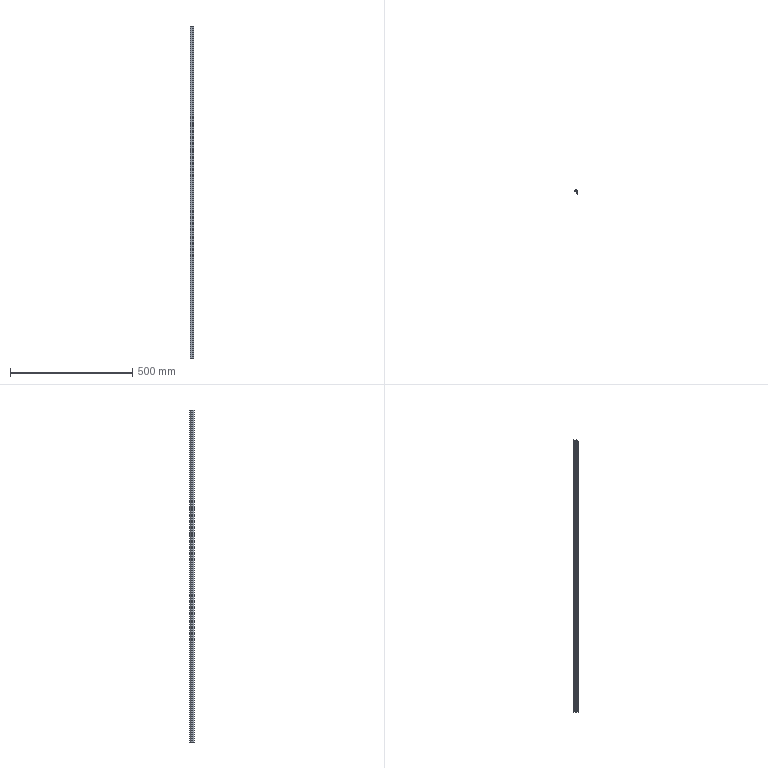Part | SolidWorks | features BaseBody 1, ICE 1, MoveFace 1 | 1 solid | 27 faces | box 14 x 20.3 x 1358 mm | volume 69144 mm3 | plane 20 | cylinder 7 | commonest cylinder face diameters 0.387 x2 0.8 x2 0.4 x1 20 x1 22 x1
STEP:
#1=CARTESIAN_POINT('',(-5.304,-0.625,200.));
#2=VERTEX_POINT('',#1);
#3=CARTESIAN_POINT('',(-5.449,-0.8125,200.));
#4=VERTEX_POINT('',#3);
#5=CARTESIAN_POINT('',(-5.255,-0.8125,200.));
#6=DIRECTION('',(0.,0.,1.));
#7=DIRECTION('',(-1.,0.,0.));
#8=AXIS2_PLACEMENT_3D('',#5,#6,#7);
#9=CIRCLE('',#8,0.1937);
#10=EDGE_CURVE('',#2,#4,#9,.T.);
#11=ORIENTED_EDGE('',*,*,#10,.T.);
#12=CARTESIAN_POINT('',(-5.449,-0.8125,-1158.));
#13=VERTEX_POINT('',#12);
#14=CARTESIAN_POINT('',(-5.449,-0.8125,230.));
#15=DIRECTION('',(0.,0.,-1.));
#16=VECTOR('',#15,1000.);
#17=LINE('',#14,#16);
#18=EDGE_CURVE('',#4,#13,#17,.T.);
#19=ORIENTED_EDGE('',*,*,#18,.T.);
#20=CARTESIAN_POINT('',(-5.304,-0.625,-1158.));
#21=VERTEX_POINT('',#20);
#22=CARTESIAN_POINT('',(-5.255,-0.8125,-1158.));
#23=DIRECTION('',(0.,0.,-1.));
#24=DIRECTION('',(1.,0.,0.));
#25=AXIS2_PLACEMENT_3D('',#22,#23,#24);
#26=CIRCLE('',#25,0.1937);
#27=EDGE_CURVE('',#13,#21,#26,.T.);
#28=ORIENTED_EDGE('',*,*,#27,.T.);
#29=CARTESIAN_POINT('',(-5.304,-0.625,230.));
#30=DIRECTION('',(0.,0.,-1.));
#31=VECTOR('',#30,1000.);
#32=LINE('',#29,#31);
#33=EDGE_CURVE('',#2,#21,#32,.T.);
#34=ORIENTED_EDGE('',*,*,#33,.F.);
#35=EDGE_LOOP('',(#11,#19,#28,#34));
#36=FACE_OUTER_BOUND('',#35,.T.);
#37=CARTESIAN_POINT('',(-5.255,-0.8125,230.));
#38=DIRECTION('',(0.,0.,-1.));
#39=DIRECTION('',(-1.,0.,0.));
#40=AXIS2_PLACEMENT_3D('',#37,#38,#39);
#41=CYLINDRICAL_SURFACE('',#40,0.1937);
#42=ADVANCED_FACE('',(#36),#41,.F.);
#43=CARTESIAN_POINT('',(5.,-1.,-1158.));
#44=VERTEX_POINT('',#43);
#45=CARTESIAN_POINT('',(5.,-14.3,-1158.));
#46=VERTEX_POINT('',#45);
#47=CARTESIAN_POINT('',(5.,29.623,-1158.));
#48=DIRECTION('',(0.,-1.,0.));
#49=VECTOR('',#48,1000.);
#50=LINE('',#47,#49);
#51=EDGE_CURVE('',#44,#46,#50,.T.);
#52=ORIENTED_EDGE('',*,*,#51,.F.);
#53=CARTESIAN_POINT('',(5.,-1.,200.));
#54=VERTEX_POINT('',#53);
#55=CARTESIAN_POINT('',(5.,-1.,230.));
#56=DIRECTION('',(0.,0.,-1.));
#57=VECTOR('',#56,1000.);
#58=LINE('',#55,#57);
#59=EDGE_CURVE('',#54,#44,#58,.T.);
#60=ORIENTED_EDGE('',*,*,#59,.F.);
#61=CARTESIAN_POINT('',(5.,-14.3,200.));
#62=VERTEX_POINT('',#61);
#63=CARTESIAN_POINT('',(5.,-14.3,200.));
#64=DIRECTION('',(0.,1.,0.));
#65=VECTOR('',#64,1000.);
#66=LINE('',#63,#65);
#67=EDGE_CURVE('',#62,#54,#66,.T.);
#68=ORIENTED_EDGE('',*,*,#67,.F.);
#69=CARTESIAN_POINT('',(5.,-14.3,230.));
#70=DIRECTION('',(0.,0.,1.));
#71=VECTOR('',#70,1000.);
#72=LINE('',#69,#71);
#73=EDGE_CURVE('',#46,#62,#72,.T.);
#74=ORIENTED_EDGE('',*,*,#73,.F.);
#75=EDGE_LOOP('',(#52,#60,#68,#74));
#76=FACE_OUTER_BOUND('',#75,.T.);
#77=CARTESIAN_POINT('',(5.,-14.3,230.));
#78=DIRECTION('',(-1.,0.,0.));
#79=DIRECTION('',(0.,0.,1.));
#80=AXIS2_PLACEMENT_3D('',#77,#78,#79);
#81=PLANE('',#80);
#82=ADVANCED_FACE('',(#76),#81,.F.);
#83=CARTESIAN_POINT('',(-9.,-2.,-1158.));
#84=VERTEX_POINT('',#83);
#85=CARTESIAN_POINT('',(-9.,-2.,200.));
#86=VERTEX_POINT('',#85);
#87=CARTESIAN_POINT('',(-9.,-2.,230.));
#88=DIRECTION('',(0.,0.,1.));
#89=VECTOR('',#88,1000.);
#90=LINE('',#87,#89);
#91=EDGE_CURVE('',#84,#86,#90,.T.);
#92=ORIENTED_EDGE('',*,*,#91,.F.);
#93=CARTESIAN_POINT('',(0.9,-2.,-1158.));
#94=VERTEX_POINT('',#93);
#95=CARTESIAN_POINT('',(5.,-2.,-1158.));
#96=DIRECTION('',(-1.,0.,0.));
#97=VECTOR('',#96,1000.);
#98=LINE('',#95,#97);
#99=EDGE_CURVE('',#94,#84,#98,.T.);
#100=ORIENTED_EDGE('',*,*,#99,.F.);
#101=CARTESIAN_POINT('',(0.9,-2.,200.));
#102=VERTEX_POINT('',#101);
#103=CARTESIAN_POINT('',(0.9,-2.,230.));
#104=DIRECTION('',(0.,0.,-1.));
#105=VECTOR('',#104,1000.);
#106=LINE('',#103,#105);
#107=EDGE_CURVE('',#102,#94,#106,.T.);
#108=ORIENTED_EDGE('',*,*,#107,.F.);
#109=CARTESIAN_POINT('',(5.,-2.,200.));
#110=DIRECTION('',(1.,0.,0.));
#111=VECTOR('',#110,1000.);
#112=LINE('',#109,#111);
#113=EDGE_CURVE('',#86,#102,#112,.T.);
#114=ORIENTED_EDGE('',*,*,#113,.F.);
#115=EDGE_LOOP('',(#92,#100,#108,#114));
#116=FACE_OUTER_BOUND('',#115,.T.);
#117=CARTESIAN_POINT('',(-9.,-2.,230.));
#118=DIRECTION('',(0.,1.,0.));
#119=DIRECTION('',(0.,0.,1.));
#120=AXIS2_PLACEMENT_3D('',#117,#118,#119);
#121=PLANE('',#120);
#122=ADVANCED_FACE('',(#116),#121,.F.);
#123=CARTESIAN_POINT('',(4.,-6.,200.));
#124=VERTEX_POINT('',#123);
#125=CARTESIAN_POINT('',(4.,-3.,200.));
#126=VERTEX_POINT('',#125);
#127=CARTESIAN_POINT('',(4.,29.623,200.));
#128=DIRECTION('',(0.,1.,0.));
#129=VECTOR('',#128,1000.);
#130=LINE('',#127,#129);
#131=EDGE_CURVE('',#124,#126,#130,.T.);
#132=ORIENTED_EDGE('',*,*,#131,.F.);
#133=CARTESIAN_POINT('',(1.,-6.,200.));
#134=VERTEX_POINT('',#133);
#135=CARTESIAN_POINT('',(5.,-6.,200.));
#136=DIRECTION('',(1.,0.,0.));
#137=VECTOR('',#136,1000.);
#138=LINE('',#135,#137);
#139=EDGE_CURVE('',#134,#124,#138,.T.);
#140=ORIENTED_EDGE('',*,*,#139,.F.);
#141=CARTESIAN_POINT('',(1.,-6.7,200.));
#142=VERTEX_POINT('',#141);
#143=CARTESIAN_POINT('',(1.,-6.,200.));
#144=DIRECTION('',(0.,-1.,0.));
#145=VECTOR('',#144,1000.);
#146=LINE('',#143,#145);
#147=EDGE_CURVE('',#134,#142,#146,.T.);
#148=ORIENTED_EDGE('',*,*,#147,.T.);
#149=CARTESIAN_POINT('',(-1.7,-6.7,200.));
#150=VERTEX_POINT('',#149);
#151=CARTESIAN_POINT('',(5.,-6.7,200.));
#152=DIRECTION('',(1.,0.,0.));
#153=VECTOR('',#152,1000.);
#154=LINE('',#151,#153);
#155=EDGE_CURVE('',#150,#142,#154,.T.);
#156=ORIENTED_EDGE('',*,*,#155,.F.);
#157=CARTESIAN_POINT('',(-1.7,-7.7,200.));
#158=VERTEX_POINT('',#157);
#159=CARTESIAN_POINT('',(-1.7,-6.7,200.));
#160=DIRECTION('',(0.,-1.,0.));
#161=VECTOR('',#160,1000.);
#162=LINE('',#159,#161);
#163=EDGE_CURVE('',#150,#158,#162,.T.);
#164=ORIENTED_EDGE('',*,*,#163,.T.);
#165=CARTESIAN_POINT('',(4.,-7.7,200.));
#166=VERTEX_POINT('',#165);
#167=CARTESIAN_POINT('',(5.,-7.7,200.));
#168=DIRECTION('',(-1.,0.,0.));
#169=VECTOR('',#168,1000.);
#170=LINE('',#167,#169);
#171=EDGE_CURVE('',#166,#158,#170,.T.);
#172=ORIENTED_EDGE('',*,*,#171,.F.);
#173=CARTESIAN_POINT('',(4.,-14.3,200.));
#174=VERTEX_POINT('',#173);
#175=CARTESIAN_POINT('',(4.,29.623,200.));
#176=DIRECTION('',(0.,1.,0.));
#177=VECTOR('',#176,1000.);
#178=LINE('',#175,#177);
#179=EDGE_CURVE('',#174,#166,#178,.T.);
#180=ORIENTED_EDGE('',*,*,#179,.F.);
#181=CARTESIAN_POINT('',(5.,-14.3,200.));
#182=DIRECTION('',(-1.,0.,0.));
#183=VECTOR('',#182,1000.);
#184=LINE('',#181,#183);
#185=EDGE_CURVE('',#62,#174,#184,.T.);
#186=ORIENTED_EDGE('',*,*,#185,.F.);
#187=ORIENTED_EDGE('',*,*,#67,.T.);
#188=CARTESIAN_POINT('',(-5.207,-1.,200.));
#189=VERTEX_POINT('',#188);
#190=CARTESIAN_POINT('',(5.,-1.,200.));
#191=DIRECTION('',(1.,0.,0.));
#192=VECTOR('',#191,1000.);
#193=LINE('',#190,#192);
#194=EDGE_CURVE('',#189,#54,#193,.T.);
#195=ORIENTED_EDGE('',*,*,#194,.F.);
#196=CARTESIAN_POINT('',(-5.255,-0.8125,200.));
#197=DIRECTION('',(0.,0.,1.));
#198=DIRECTION('',(-1.,0.,0.));
#199=AXIS2_PLACEMENT_3D('',#196,#197,#198);
#200=CIRCLE('',#199,0.1937);
#201=EDGE_CURVE('',#4,#189,#200,.T.);
#202=ORIENTED_EDGE('',*,*,#201,.F.);
#203=ORIENTED_EDGE('',*,*,#10,.F.);
#204=CARTESIAN_POINT('',(-1.368,3.063,200.));
#205=VERTEX_POINT('',#204);
#206=CARTESIAN_POINT('',(-10.628,9.,200.));
#207=DIRECTION('',(0.,0.,1.));
#208=DIRECTION('',(-1.,0.,0.));
#209=AXIS2_PLACEMENT_3D('',#206,#207,#208);
#210=CIRCLE('',#209,11.);
#211=EDGE_CURVE('',#2,#205,#210,.T.);
#212=ORIENTED_EDGE('',*,*,#211,.T.);
#213=CARTESIAN_POINT('',(-1.,2.955,200.));
#214=VERTEX_POINT('',#213);
#215=CARTESIAN_POINT('',(-1.2,2.955,200.));
#216=DIRECTION('',(0.,0.,1.));
#217=DIRECTION('',(-1.,0.,0.));
#218=AXIS2_PLACEMENT_3D('',#215,#216,#217);
#219=CIRCLE('',#218,0.2);
#220=EDGE_CURVE('',#214,#205,#219,.T.);
#221=ORIENTED_EDGE('',*,*,#220,.F.);
#222=CARTESIAN_POINT('',(-1.,1.5,200.));
#223=VERTEX_POINT('',#222);
#224=CARTESIAN_POINT('',(-1.,2.955,200.));
#225=DIRECTION('',(0.,1.,0.));
#226=VECTOR('',#225,1000.);
#227=LINE('',#224,#226);
#228=EDGE_CURVE('',#223,#214,#227,.T.);
#229=ORIENTED_EDGE('',*,*,#228,.F.);
#230=CARTESIAN_POINT('',(0.,1.5,200.));
#231=VERTEX_POINT('',#230);
#232=CARTESIAN_POINT('',(-1.,1.5,200.));
#233=DIRECTION('',(-1.,0.,0.));
#234=VECTOR('',#233,1000.);
#235=LINE('',#232,#234);
#236=EDGE_CURVE('',#231,#223,#235,.T.);
#237=ORIENTED_EDGE('',*,*,#236,.F.);
#238=CARTESIAN_POINT('',(0.,6.,200.));
#239=VERTEX_POINT('',#238);
#240=CARTESIAN_POINT('',(0.,1.5,200.));
#241=DIRECTION('',(0.,-1.,0.));
#242=VECTOR('',#241,1000.);
#243=LINE('',#240,#242);
#244=EDGE_CURVE('',#239,#231,#243,.T.);
#245=ORIENTED_EDGE('',*,*,#244,.F.);
#246=CARTESIAN_POINT('',(-0.8,6.,200.));
#247=VERTEX_POINT('',#246);
#248=CARTESIAN_POINT('',(0.,6.,200.));
#249=DIRECTION('',(1.,0.,0.));
#250=VECTOR('',#249,1000.);
#251=LINE('',#248,#250);
#252=EDGE_CURVE('',#247,#239,#251,.T.);
#253=ORIENTED_EDGE('',*,*,#252,.F.);
#254=CARTESIAN_POINT('',(-1.178,5.731,200.));
#255=VERTEX_POINT('',#254);
#256=CARTESIAN_POINT('',(-0.8,5.6,200.));
#257=DIRECTION('',(0.,0.,1.));
#258=DIRECTION('',(-1.,0.,0.));
#259=AXIS2_PLACEMENT_3D('',#256,#257,#258);
#260=CIRCLE('',#259,0.4);
#261=EDGE_CURVE('',#247,#255,#260,.T.);
#262=ORIENTED_EDGE('',*,*,#261,.T.);
#263=CARTESIAN_POINT('',(-8.678,-0.8077,200.));
#264=VERTEX_POINT('',#263);
#265=CARTESIAN_POINT('',(-10.628,9.,200.));
#266=DIRECTION('',(0.,0.,1.));
#267=DIRECTION('',(-1.,0.,0.));
#268=AXIS2_PLACEMENT_3D('',#265,#266,#267);
#269=CIRCLE('',#268,10.);
#270=EDGE_CURVE('',#264,#255,#269,.T.);
#271=ORIENTED_EDGE('',*,*,#270,.F.);
#272=CARTESIAN_POINT('',(-9.,-1.2,200.));
#273=VERTEX_POINT('',#272);
#274=CARTESIAN_POINT('',(-8.6,-1.2,200.));
#275=DIRECTION('',(0.,0.,1.));
#276=DIRECTION('',(-1.,0.,0.));
#277=AXIS2_PLACEMENT_3D('',#274,#275,#276);
#278=CIRCLE('',#277,0.4);
#279=EDGE_CURVE('',#264,#273,#278,.T.);
#280=ORIENTED_EDGE('',*,*,#279,.T.);
#281=CARTESIAN_POINT('',(-9.,8.,200.));
#282=DIRECTION('',(0.,-1.,0.));
#283=VECTOR('',#282,1000.);
#284=LINE('',#281,#283);
#285=EDGE_CURVE('',#273,#86,#284,.T.);
#286=ORIENTED_EDGE('',*,*,#285,.T.);
#287=ORIENTED_EDGE('',*,*,#113,.T.);
#288=CARTESIAN_POINT('',(0.9,-3.,200.));
#289=VERTEX_POINT('',#288);
#290=CARTESIAN_POINT('',(0.9,29.623,200.));
#291=DIRECTION('',(0.,1.,0.));
#292=VECTOR('',#291,1000.);
#293=LINE('',#290,#292);
#294=EDGE_CURVE('',#289,#102,#293,.T.);
#295=ORIENTED_EDGE('',*,*,#294,.F.);
#296=CARTESIAN_POINT('',(5.,-3.,200.));
#297=DIRECTION('',(-1.,0.,0.));
#298=VECTOR('',#297,1000.);
#299=LINE('',#296,#298);
#300=EDGE_CURVE('',#126,#289,#299,.T.);
#301=ORIENTED_EDGE('',*,*,#300,.F.);
#302=EDGE_LOOP('',(#132,#140,#148,#156,#164,#172,#180,#186,#187,#195,#202,#203,#212,#221,#229,#237,#245,#253,#262,#271,#280,#286,#287,#295,#301));
#303=FACE_OUTER_BOUND('',#302,.T.);
#304=CARTESIAN_POINT('',(5.,29.623,200.));
#305=DIRECTION('',(0.,0.,-1.));
#306=DIRECTION('',(-1.,0.,0.));
#307=AXIS2_PLACEMENT_3D('',#304,#305,#306);
#308=PLANE('',#307);
#309=ADVANCED_FACE('',(#303),#308,.F.);
#310=ORIENTED_EDGE('',*,*,#185,.T.);
#311=CARTESIAN_POINT('',(4.,-14.3,-1158.));
#312=VERTEX_POINT('',#311);
#313=CARTESIAN_POINT('',(4.,-14.3,230.));
#314=DIRECTION('',(0.,0.,1.));
#315=VECTOR('',#314,1000.);
#316=LINE('',#313,#315);
#317=EDGE_CURVE('',#312,#174,#316,.T.);
#318=ORIENTED_EDGE('',*,*,#317,.F.);
#319=CARTESIAN_POINT('',(5.,-14.3,-1158.));
#320=DIRECTION('',(-1.,0.,0.));
#321=VECTOR('',#320,1000.);
#322=LINE('',#319,#321);
#323=EDGE_CURVE('',#46,#312,#322,.T.);
#324=ORIENTED_EDGE('',*,*,#323,.F.);
#325=ORIENTED_EDGE('',*,*,#73,.T.);
#326=EDGE_LOOP('',(#310,#318,#324,#325));
#327=FACE_OUTER_BOUND('',#326,.T.);
#328=CARTESIAN_POINT('',(4.,-14.3,230.));
#329=DIRECTION('',(0.,1.,0.));
#330=DIRECTION('',(0.,0.,1.));
#331=AXIS2_PLACEMENT_3D('',#328,#329,#330);
#332=PLANE('',#331);
#333=ADVANCED_FACE('',(#327),#332,.F.);
#334=ORIENTED_EDGE('',*,*,#51,.T.);
#335=ORIENTED_EDGE('',*,*,#323,.T.);
#336=CARTESIAN_POINT('',(4.,-7.7,-1158.));
#337=VERTEX_POINT('',#336);
#338=CARTESIAN_POINT('',(4.,-7.7,-1158.));
#339=DIRECTION('',(0.,-1.,0.));
#340=VECTOR('',#339,1000.);
#341=LINE('',#338,#340);
#342=EDGE_CURVE('',#337,#312,#341,.T.);
#343=ORIENTED_EDGE('',*,*,#342,.F.);
#344=CARTESIAN_POINT('',(-1.7,-7.7,-1158.));
#345=VERTEX_POINT('',#344);
#346=CARTESIAN_POINT('',(-1.7,-7.7,-1158.));
#347=DIRECTION('',(1.,0.,0.));
#348=VECTOR('',#347,1000.);
#349=LINE('',#346,#348);
#350=EDGE_CURVE('',#345,#337,#349,.T.);
#351=ORIENTED_EDGE('',*,*,#350,.F.);
#352=CARTESIAN_POINT('',(-1.7,-6.7,-1158.));
#353=VERTEX_POINT('',#352);
#354=CARTESIAN_POINT('',(-1.7,29.623,-1158.));
#355=DIRECTION('',(0.,1.,0.));
#356=VECTOR('',#355,1000.);
#357=LINE('',#354,#356);
#358=EDGE_CURVE('',#345,#353,#357,.T.);
#359=ORIENTED_EDGE('',*,*,#358,.T.);
#360=CARTESIAN_POINT('',(1.,-6.7,-1158.));
#361=VERTEX_POINT('',#360);
#362=CARTESIAN_POINT('',(1.,-6.7,-1158.));
#363=DIRECTION('',(-1.,0.,0.));
#364=VECTOR('',#363,1000.);
#365=LINE('',#362,#364);
#366=EDGE_CURVE('',#361,#353,#365,.T.);
#367=ORIENTED_EDGE('',*,*,#366,.F.);
#368=CARTESIAN_POINT('',(1.,-6.,-1158.));
#369=VERTEX_POINT('',#368);
#370=CARTESIAN_POINT('',(1.,29.623,-1158.));
#371=DIRECTION('',(0.,1.,0.));
#372=VECTOR('',#371,1000.);
#373=LINE('',#370,#372);
#374=EDGE_CURVE('',#361,#369,#373,.T.);
#375=ORIENTED_EDGE('',*,*,#374,.T.);
#376=CARTESIAN_POINT('',(4.,-6.,-1158.));
#377=VERTEX_POINT('',#376);
#378=CARTESIAN_POINT('',(4.,-6.,-1158.));
#379=DIRECTION('',(-1.,0.,0.));
#380=VECTOR('',#379,1000.);
#381=LINE('',#378,#380);
#382=EDGE_CURVE('',#377,#369,#381,.T.);
#383=ORIENTED_EDGE('',*,*,#382,.F.);
#384=CARTESIAN_POINT('',(4.,-3.,-1158.));
#385=VERTEX_POINT('',#384);
#386=CARTESIAN_POINT('',(4.,-3.,-1158.));
#387=DIRECTION('',(0.,-1.,0.));
#388=VECTOR('',#387,1000.);
#389=LINE('',#386,#388);
#390=EDGE_CURVE('',#385,#377,#389,.T.);
#391=ORIENTED_EDGE('',*,*,#390,.F.);
#392=CARTESIAN_POINT('',(0.9,-3.,-1158.));
#393=VERTEX_POINT('',#392);
#394=CARTESIAN_POINT('',(0.9,-3.,-1158.));
#395=DIRECTION('',(1.,0.,0.));
#396=VECTOR('',#395,1000.);
#397=LINE('',#394,#396);
#398=EDGE_CURVE('',#393,#385,#397,.T.);
#399=ORIENTED_EDGE('',*,*,#398,.F.);
#400=CARTESIAN_POINT('',(0.9,-2.,-1158.));
#401=DIRECTION('',(0.,-1.,0.));
#402=VECTOR('',#401,1000.);
#403=LINE('',#400,#402);
#404=EDGE_CURVE('',#94,#393,#403,.T.);
#405=ORIENTED_EDGE('',*,*,#404,.F.);
#406=ORIENTED_EDGE('',*,*,#99,.T.);
#407=CARTESIAN_POINT('',(-9.,-1.2,-1158.));
#408=VERTEX_POINT('',#407);
#409=CARTESIAN_POINT('',(-9.,-1.2,-1158.));
#410=DIRECTION('',(0.,-1.,0.));
#411=VECTOR('',#410,1000.);
#412=LINE('',#409,#411);
#413=EDGE_CURVE('',#408,#84,#412,.T.);
#414=ORIENTED_EDGE('',*,*,#413,.F.);
#415=CARTESIAN_POINT('',(-8.678,-0.8077,-1158.));
#416=VERTEX_POINT('',#415);
#417=CARTESIAN_POINT('',(-8.6,-1.2,-1158.));
#418=DIRECTION('',(0.,0.,-1.));
#419=DIRECTION('',(1.,0.,0.));
#420=AXIS2_PLACEMENT_3D('',#417,#418,#419);
#421=CIRCLE('',#420,0.4);
#422=EDGE_CURVE('',#408,#416,#421,.T.);
#423=ORIENTED_EDGE('',*,*,#422,.T.);
#424=CARTESIAN_POINT('',(-1.178,5.731,-1158.));
#425=VERTEX_POINT('',#424);
#426=CARTESIAN_POINT('',(-10.628,9.,-1158.));
#427=DIRECTION('',(0.,0.,-1.));
#428=DIRECTION('',(1.,0.,0.));
#429=AXIS2_PLACEMENT_3D('',#426,#427,#428);
#430=CIRCLE('',#429,10.);
#431=EDGE_CURVE('',#425,#416,#430,.T.);
#432=ORIENTED_EDGE('',*,*,#431,.F.);
#433=CARTESIAN_POINT('',(-0.8,6.,-1158.));
#434=VERTEX_POINT('',#433);
#435=CARTESIAN_POINT('',(-0.8,5.6,-1158.));
#436=DIRECTION('',(0.,0.,-1.));
#437=DIRECTION('',(1.,0.,0.));
#438=AXIS2_PLACEMENT_3D('',#435,#436,#437);
#439=CIRCLE('',#438,0.4);
#440=EDGE_CURVE('',#425,#434,#439,.T.);
#441=ORIENTED_EDGE('',*,*,#440,.T.);
#442=CARTESIAN_POINT('',(0.,6.,-1158.));
#443=VERTEX_POINT('',#442);
#444=CARTESIAN_POINT('',(0.,6.,-1158.));
#445=DIRECTION('',(-1.,0.,0.));
#446=VECTOR('',#445,1000.);
#447=LINE('',#444,#446);
#448=EDGE_CURVE('',#443,#434,#447,.T.);
#449=ORIENTED_EDGE('',*,*,#448,.F.);
#450=CARTESIAN_POINT('',(0.,1.5,-1158.));
#451=VERTEX_POINT('',#450);
#452=CARTESIAN_POINT('',(0.,1.5,-1158.));
#453=DIRECTION('',(0.,1.,0.));
#454=VECTOR('',#453,1000.);
#455=LINE('',#452,#454);
#456=EDGE_CURVE('',#451,#443,#455,.T.);
#457=ORIENTED_EDGE('',*,*,#456,.F.);
#458=CARTESIAN_POINT('',(-1.,1.5,-1158.));
#459=VERTEX_POINT('',#458);
#460=CARTESIAN_POINT('',(-1.,1.5,-1158.));
#461=DIRECTION('',(1.,0.,0.));
#462=VECTOR('',#461,1000.);
#463=LINE('',#460,#462);
#464=EDGE_CURVE('',#459,#451,#463,.T.);
#465=ORIENTED_EDGE('',*,*,#464,.F.);
#466=CARTESIAN_POINT('',(-1.,2.955,-1158.));
#467=VERTEX_POINT('',#466);
#468=CARTESIAN_POINT('',(-1.,2.955,-1158.));
#469=DIRECTION('',(0.,-1.,0.));
#470=VECTOR('',#469,1000.);
#471=LINE('',#468,#470);
#472=EDGE_CURVE('',#467,#459,#471,.T.);
#473=ORIENTED_EDGE('',*,*,#472,.F.);
#474=CARTESIAN_POINT('',(-1.368,3.063,-1158.));
#475=VERTEX_POINT('',#474);
#476=CARTESIAN_POINT('',(-1.2,2.955,-1158.));
#477=DIRECTION('',(0.,0.,-1.));
#478=DIRECTION('',(1.,0.,0.));
#479=AXIS2_PLACEMENT_3D('',#476,#477,#478);
#480=CIRCLE('',#479,0.2);
#481=EDGE_CURVE('',#475,#467,#480,.T.);
#482=ORIENTED_EDGE('',*,*,#481,.F.);
#483=CARTESIAN_POINT('',(-10.628,9.,-1158.));
#484=DIRECTION('',(0.,0.,-1.));
#485=DIRECTION('',(1.,0.,0.));
#486=AXIS2_PLACEMENT_3D('',#483,#484,#485);
#487=CIRCLE('',#486,11.);
#488=EDGE_CURVE('',#475,#21,#487,.T.);
#489=ORIENTED_EDGE('',*,*,#488,.T.);
#490=ORIENTED_EDGE('',*,*,#27,.F.);
#491=CARTESIAN_POINT('',(-5.207,-1.,-1158.));
#492=VERTEX_POINT('',#491);
#493=CARTESIAN_POINT('',(-5.255,-0.8125,-1158.));
#494=DIRECTION('',(0.,0.,-1.));
#495=DIRECTION('',(1.,0.,0.));
#496=AXIS2_PLACEMENT_3D('',#493,#494,#495);
#497=CIRCLE('',#496,0.1937);
#498=EDGE_CURVE('',#492,#13,#497,.T.);
#499=ORIENTED_EDGE('',*,*,#498,.F.);
#500=CARTESIAN_POINT('',(5.,-1.,-1158.));
#501=DIRECTION('',(-1.,0.,0.));
#502=VECTOR('',#501,1000.);
#503=LINE('',#500,#502);
#504=EDGE_CURVE('',#44,#492,#503,.T.);
#505=ORIENTED_EDGE('',*,*,#504,.F.);
#506=EDGE_LOOP('',(#334,#335,#343,#351,#359,#367,#375,#383,#391,#399,#405,#406,#414,#423,#432,#441,#449,#457,#465,#473,#482,#489,#490,#499,#505));
#507=FACE_OUTER_BOUND('',#506,.T.);
#508=CARTESIAN_POINT('',(5.,29.623,-1158.));
#509=DIRECTION('',(0.,0.,1.));
#510=DIRECTION('',(1.,0.,0.));
#511=AXIS2_PLACEMENT_3D('',#508,#509,#510);
#512=PLANE('',#511);
#513=ADVANCED_FACE('',(#507),#512,.F.);
#514=ORIENTED_EDGE('',*,*,#59,.T.);
#515=ORIENTED_EDGE('',*,*,#504,.T.);
#516=CARTESIAN_POINT('',(-5.207,-1.,230.));
#517=DIRECTION('',(0.,0.,-1.));
#518=VECTOR('',#517,1000.);
#519=LINE('',#516,#518);
#520=EDGE_CURVE('',#189,#492,#519,.T.);
#521=ORIENTED_EDGE('',*,*,#520,.F.);
#522=ORIENTED_EDGE('',*,*,#194,.T.);
#523=EDGE_LOOP('',(#514,#515,#521,#522));
#524=FACE_OUTER_BOUND('',#523,.T.);
#525=CARTESIAN_POINT('',(5.,-1.,230.));
#526=DIRECTION('',(0.,-1.,0.));
#527=DIRECTION('',(0.,0.,-1.));
#528=AXIS2_PLACEMENT_3D('',#525,#526,#527);
#529=PLANE('',#528);
#530=ADVANCED_FACE('',(#524),#529,.F.);
#531=CARTESIAN_POINT('',(-9.,-1.2,230.));
#532=DIRECTION('',(0.,0.,1.));
#533=VECTOR('',#532,1000.);
#534=LINE('',#531,#533);
#535=EDGE_CURVE('',#408,#273,#534,.T.);
#536=ORIENTED_EDGE('',*,*,#535,.F.);
#537=ORIENTED_EDGE('',*,*,#413,.T.);
#538=ORIENTED_EDGE('',*,*,#91,.T.);
#539=ORIENTED_EDGE('',*,*,#285,.F.);
#540=EDGE_LOOP('',(#536,#537,#538,#539));
#541=FACE_OUTER_BOUND('',#540,.T.);
#542=CARTESIAN_POINT('',(-9.,-1.2,230.));
#543=DIRECTION('',(1.,0.,0.));
#544=DIRECTION('',(0.,0.,-1.));
#545=AXIS2_PLACEMENT_3D('',#542,#543,#544);
#546=PLANE('',#545);
#547=ADVANCED_FACE('',(#541),#546,.F.);
#548=ORIENTED_EDGE('',*,*,#294,.T.);
#549=ORIENTED_EDGE('',*,*,#107,.T.);
#550=ORIENTED_EDGE('',*,*,#404,.T.);
#551=CARTESIAN_POINT('',(0.9,-3.,230.));
#552=DIRECTION('',(0.,0.,-1.));
#553=VECTOR('',#552,1000.);
#554=LINE('',#551,#553);
#555=EDGE_CURVE('',#289,#393,#554,.T.);
#556=ORIENTED_EDGE('',*,*,#555,.F.);
#557=EDGE_LOOP('',(#548,#549,#550,#556));
#558=FACE_OUTER_BOUND('',#557,.T.);
#559=CARTESIAN_POINT('',(0.9,-2.,230.));
#560=DIRECTION('',(1.,0.,0.));
#561=DIRECTION('',(0.,0.,-1.));
#562=AXIS2_PLACEMENT_3D('',#559,#560,#561);
#563=PLANE('',#562);
#564=ADVANCED_FACE('',(#558),#563,.F.);
#565=ORIENTED_EDGE('',*,*,#300,.T.);
#566=ORIENTED_EDGE('',*,*,#555,.T.);
#567=ORIENTED_EDGE('',*,*,#398,.T.);
#568=CARTESIAN_POINT('',(4.,-3.,230.));
#569=DIRECTION('',(0.,0.,-1.));
#570=VECTOR('',#569,1000.);
#571=LINE('',#568,#570);
#572=EDGE_CURVE('',#126,#385,#571,.T.);
#573=ORIENTED_EDGE('',*,*,#572,.F.);
#574=EDGE_LOOP('',(#565,#566,#567,#573));
#575=FACE_OUTER_BOUND('',#574,.T.);
#576=CARTESIAN_POINT('',(0.9,-3.,230.));
#577=DIRECTION('',(0.,1.,0.));
#578=DIRECTION('',(0.,0.,1.));
#579=AXIS2_PLACEMENT_3D('',#576,#577,#578);
#580=PLANE('',#579);
#581=ADVANCED_FACE('',(#575),#580,.F.);
#582=ORIENTED_EDGE('',*,*,#131,.T.);
#583=ORIENTED_EDGE('',*,*,#572,.T.);
#584=ORIENTED_EDGE('',*,*,#390,.T.);
#585=CARTESIAN_POINT('',(4.,-6.,230.));
#586=DIRECTION('',(0.,0.,-1.));
#587=VECTOR('',#586,1000.);
#588=LINE('',#585,#587);
#589=EDGE_CURVE('',#124,#377,#588,.T.);
#590=ORIENTED_EDGE('',*,*,#589,.F.);
#591=EDGE_LOOP('',(#582,#583,#584,#590));
#592=FACE_OUTER_BOUND('',#591,.T.);
#593=CARTESIAN_POINT('',(4.,-3.,230.));
#594=DIRECTION('',(1.,0.,0.));
#595=DIRECTION('',(0.,0.,-1.));
#596=AXIS2_PLACEMENT_3D('',#593,#594,#595);
#597=PLANE('',#596);
#598=ADVANCED_FACE('',(#592),#597,.F.);
#599=ORIENTED_EDGE('',*,*,#139,.T.);
#600=ORIENTED_EDGE('',*,*,#589,.T.);
#601=ORIENTED_EDGE('',*,*,#382,.T.);
#602=CARTESIAN_POINT('',(1.,-6.,230.));
#603=DIRECTION('',(0.,0.,-1.));
#604=VECTOR('',#603,1000.);
#605=LINE('',#602,#604);
#606=EDGE_CURVE('',#134,#369,#605,.T.);
#607=ORIENTED_EDGE('',*,*,#606,.F.);
#608=EDGE_LOOP('',(#599,#600,#601,#607));
#609=FACE_OUTER_BOUND('',#608,.T.);
#610=CARTESIAN_POINT('',(4.,-6.,230.));
#611=DIRECTION('',(0.,-1.,0.));
#612=DIRECTION('',(0.,0.,-1.));
#613=AXIS2_PLACEMENT_3D('',#610,#611,#612);
#614=PLANE('',#613);
#615=ADVANCED_FACE('',(#609),#614,.F.);
#616=ORIENTED_EDGE('',*,*,#155,.T.);
#617=CARTESIAN_POINT('',(1.,-6.7,230.));
#618=DIRECTION('',(0.,0.,1.));
#619=VECTOR('',#618,1000.);
#620=LINE('',#617,#619);
#621=EDGE_CURVE('',#361,#142,#620,.T.);
#622=ORIENTED_EDGE('',*,*,#621,.F.);
#623=ORIENTED_EDGE('',*,*,#366,.T.);
#624=CARTESIAN_POINT('',(-1.7,-6.7,230.));
#625=DIRECTION('',(0.,0.,-1.));
#626=VECTOR('',#625,1000.);
#627=LINE('',#624,#626);
#628=EDGE_CURVE('',#150,#353,#627,.T.);
#629=ORIENTED_EDGE('',*,*,#628,.F.);
#630=EDGE_LOOP('',(#616,#622,#623,#629));
#631=FACE_OUTER_BOUND('',#630,.T.);
#632=CARTESIAN_POINT('',(1.,-6.7,230.));
#633=DIRECTION('',(0.,-1.,0.));
#634=DIRECTION('',(0.,0.,-1.));
#635=AXIS2_PLACEMENT_3D('',#632,#633,#634);
#636=PLANE('',#635);
#637=ADVANCED_FACE('',(#631),#636,.F.);
#638=ORIENTED_EDGE('',*,*,#171,.T.);
#639=CARTESIAN_POINT('',(-1.7,-7.7,230.));
#640=DIRECTION('',(0.,0.,1.));
#641=VECTOR('',#640,1000.);
#642=LINE('',#639,#641);
#643=EDGE_CURVE('',#345,#158,#642,.T.);
#644=ORIENTED_EDGE('',*,*,#643,.F.);
#645=ORIENTED_EDGE('',*,*,#350,.T.);
#646=CARTESIAN_POINT('',(4.,-7.7,230.));
#647=DIRECTION('',(0.,0.,-1.));
#648=VECTOR('',#647,1000.);
#649=LINE('',#646,#648);
#650=EDGE_CURVE('',#166,#337,#649,.T.);
#651=ORIENTED_EDGE('',*,*,#650,.F.);
#652=EDGE_LOOP('',(#638,#644,#645,#651));
#653=FACE_OUTER_BOUND('',#652,.T.);
#654=CARTESIAN_POINT('',(-1.7,-7.7,230.));
#655=DIRECTION('',(0.,1.,0.));
#656=DIRECTION('',(0.,0.,1.));
#657=AXIS2_PLACEMENT_3D('',#654,#655,#656);
#658=PLANE('',#657);
#659=ADVANCED_FACE('',(#653),#658,.F.);
#660=ORIENTED_EDGE('',*,*,#179,.T.);
#661=ORIENTED_EDGE('',*,*,#650,.T.);
#662=ORIENTED_EDGE('',*,*,#342,.T.);
#663=ORIENTED_EDGE('',*,*,#317,.T.);
#664=EDGE_LOOP('',(#660,#661,#662,#663));
#665=FACE_OUTER_BOUND('',#664,.T.);
#666=CARTESIAN_POINT('',(4.,-7.7,230.));
#667=DIRECTION('',(1.,0.,0.));
#668=DIRECTION('',(0.,0.,-1.));
#669=AXIS2_PLACEMENT_3D('',#666,#667,#668);
#670=PLANE('',#669);
#671=ADVANCED_FACE('',(#665),#670,.F.);
#672=ORIENTED_EDGE('',*,*,#18,.F.);
#673=ORIENTED_EDGE('',*,*,#201,.T.);
#674=ORIENTED_EDGE('',*,*,#520,.T.);
#675=ORIENTED_EDGE('',*,*,#498,.T.);
#676=EDGE_LOOP('',(#672,#673,#674,#675));
#677=FACE_OUTER_BOUND('',#676,.T.);
#678=CARTESIAN_POINT('',(-5.255,-0.8125,230.));
#679=DIRECTION('',(0.,0.,-1.));
#680=DIRECTION('',(-1.,0.,0.));
#681=AXIS2_PLACEMENT_3D('',#678,#679,#680);
#682=CYLINDRICAL_SURFACE('',#681,0.1937);
#683=ADVANCED_FACE('',(#677),#682,.F.);
#684=CARTESIAN_POINT('',(-1.,2.955,230.));
#685=DIRECTION('',(0.,0.,1.));
#686=VECTOR('',#685,1000.);
#687=LINE('',#684,#686);
#688=EDGE_CURVE('',#467,#214,#687,.T.);
#689=ORIENTED_EDGE('',*,*,#688,.F.);
#690=ORIENTED_EDGE('',*,*,#472,.T.);
#691=CARTESIAN_POINT('',(-1.,1.5,230.));
#692=DIRECTION('',(0.,0.,-1.));
#693=VECTOR('',#692,1000.);
#694=LINE('',#691,#693);
#695=EDGE_CURVE('',#223,#459,#694,.T.);
#696=ORIENTED_EDGE('',*,*,#695,.F.);
#697=ORIENTED_EDGE('',*,*,#228,.T.);
#698=EDGE_LOOP('',(#689,#690,#696,#697));
#699=FACE_OUTER_BOUND('',#698,.T.);
#700=CARTESIAN_POINT('',(-1.,2.955,230.));
#701=DIRECTION('',(1.,0.,0.));
#702=DIRECTION('',(0.,0.,-1.));
#703=AXIS2_PLACEMENT_3D('',#700,#701,#702);
#704=PLANE('',#703);
#705=ADVANCED_FACE('',(#699),#704,.F.);
#706=ORIENTED_EDGE('',*,*,#488,.F.);
#707=CARTESIAN_POINT('',(-1.368,3.063,230.));
#708=DIRECTION('',(0.,0.,1.));
#709=VECTOR('',#708,1000.);
#710=LINE('',#707,#709);
#711=EDGE_CURVE('',#475,#205,#710,.T.);
#712=ORIENTED_EDGE('',*,*,#711,.T.);
#713=ORIENTED_EDGE('',*,*,#211,.F.);
#714=ORIENTED_EDGE('',*,*,#33,.T.);
#715=EDGE_LOOP('',(#706,#712,#713,#714));
#716=FACE_OUTER_BOUND('',#715,.T.);
#717=CARTESIAN_POINT('',(-10.628,9.,230.));
#718=DIRECTION('',(0.,0.,-1.));
#719=DIRECTION('',(-1.,0.,0.));
#720=AXIS2_PLACEMENT_3D('',#717,#718,#719);
#721=CYLINDRICAL_SURFACE('',#720,11.);
#722=ADVANCED_FACE('',(#716),#721,.T.);
#723=CARTESIAN_POINT('',(-1.178,5.731,230.));
#724=DIRECTION('',(0.,0.,1.));
#725=VECTOR('',#724,1000.);
#726=LINE('',#723,#725);
#727=EDGE_CURVE('',#425,#255,#726,.T.);
#728=ORIENTED_EDGE('',*,*,#727,.F.);
#729=ORIENTED_EDGE('',*,*,#431,.T.);
#730=CARTESIAN_POINT('',(-8.678,-0.8077,230.));
#731=DIRECTION('',(0.,0.,-1.));
#732=VECTOR('',#731,1000.);
#733=LINE('',#730,#732);
#734=EDGE_CURVE('',#264,#416,#733,.T.);
#735=ORIENTED_EDGE('',*,*,#734,.F.);
#736=ORIENTED_EDGE('',*,*,#270,.T.);
#737=EDGE_LOOP('',(#728,#729,#735,#736));
#738=FACE_OUTER_BOUND('',#737,.T.);
#739=CARTESIAN_POINT('',(-10.628,9.,230.));
#740=DIRECTION('',(0.,0.,-1.));
#741=DIRECTION('',(-1.,0.,0.));
#742=AXIS2_PLACEMENT_3D('',#739,#740,#741);
#743=CYLINDRICAL_SURFACE('',#742,10.);
#744=ADVANCED_FACE('',(#738),#743,.F.);
#745=CARTESIAN_POINT('',(0.,1.5,230.));
#746=DIRECTION('',(0.,0.,1.));
#747=VECTOR('',#746,1000.);
#748=LINE('',#745,#747);
#749=EDGE_CURVE('',#451,#231,#748,.T.);
#750=ORIENTED_EDGE('',*,*,#749,.F.);
#751=ORIENTED_EDGE('',*,*,#456,.T.);
#752=CARTESIAN_POINT('',(0.,6.,230.));
#753=DIRECTION('',(0.,0.,-1.));
#754=VECTOR('',#753,1000.);
#755=LINE('',#752,#754);
#756=EDGE_CURVE('',#239,#443,#755,.T.);
#757=ORIENTED_EDGE('',*,*,#756,.F.);
#758=ORIENTED_EDGE('',*,*,#244,.T.);
#759=EDGE_LOOP('',(#750,#751,#757,#758));
#760=FACE_OUTER_BOUND('',#759,.T.);
#761=CARTESIAN_POINT('',(0.,1.5,230.));
#762=DIRECTION('',(-1.,0.,0.));
#763=DIRECTION('',(0.,0.,1.));
#764=AXIS2_PLACEMENT_3D('',#761,#762,#763);
#765=PLANE('',#764);
#766=ADVANCED_FACE('',(#760),#765,.F.);
#767=ORIENTED_EDGE('',*,*,#422,.F.);
#768=ORIENTED_EDGE('',*,*,#535,.T.);
#769=ORIENTED_EDGE('',*,*,#279,.F.);
#770=ORIENTED_EDGE('',*,*,#734,.T.);
#771=EDGE_LOOP('',(#767,#768,#769,#770));
#772=FACE_OUTER_BOUND('',#771,.T.);
#773=CARTESIAN_POINT('',(-8.6,-1.2,230.));
#774=DIRECTION('',(0.,0.,-1.));
#775=DIRECTION('',(-1.,0.,0.));
#776=AXIS2_PLACEMENT_3D('',#773,#774,#775);
#777=CYLINDRICAL_SURFACE('',#776,0.4);
#778=ADVANCED_FACE('',(#772),#777,.T.);
#779=ORIENTED_EDGE('',*,*,#147,.F.);
#780=ORIENTED_EDGE('',*,*,#606,.T.);
#781=ORIENTED_EDGE('',*,*,#374,.F.);
#782=ORIENTED_EDGE('',*,*,#621,.T.);
#783=EDGE_LOOP('',(#779,#780,#781,#782));
#784=FACE_OUTER_BOUND('',#783,.T.);
#785=CARTESIAN_POINT('',(1.,-6.,230.));
#786=DIRECTION('',(1.,0.,0.));
#787=DIRECTION('',(0.,0.,-1.));
#788=AXIS2_PLACEMENT_3D('',#785,#786,#787);
#789=PLANE('',#788);
#790=ADVANCED_FACE('',(#784),#789,.F.);
#791=ORIENTED_EDGE('',*,*,#163,.F.);
#792=ORIENTED_EDGE('',*,*,#628,.T.);
#793=ORIENTED_EDGE('',*,*,#358,.F.);
#794=ORIENTED_EDGE('',*,*,#643,.T.);
#795=EDGE_LOOP('',(#791,#792,#793,#794));
#796=FACE_OUTER_BOUND('',#795,.T.);
#797=CARTESIAN_POINT('',(-1.7,-6.7,230.));
#798=DIRECTION('',(1.,0.,0.));
#799=DIRECTION('',(0.,0.,-1.));
#800=AXIS2_PLACEMENT_3D('',#797,#798,#799);
#801=PLANE('',#800);
#802=ADVANCED_FACE('',(#796),#801,.F.);
#803=ORIENTED_EDGE('',*,*,#711,.F.);
#804=ORIENTED_EDGE('',*,*,#481,.T.);
#805=ORIENTED_EDGE('',*,*,#688,.T.);
#806=ORIENTED_EDGE('',*,*,#220,.T.);
#807=EDGE_LOOP('',(#803,#804,#805,#806));
#808=FACE_OUTER_BOUND('',#807,.T.);
#809=CARTESIAN_POINT('',(-1.2,2.955,230.));
#810=DIRECTION('',(0.,0.,-1.));
#811=DIRECTION('',(-1.,0.,0.));
#812=AXIS2_PLACEMENT_3D('',#809,#810,#811);
#813=CYLINDRICAL_SURFACE('',#812,0.2);
#814=ADVANCED_FACE('',(#808),#813,.F.);
#815=ORIENTED_EDGE('',*,*,#695,.T.);
#816=ORIENTED_EDGE('',*,*,#464,.T.);
#817=ORIENTED_EDGE('',*,*,#749,.T.);
#818=ORIENTED_EDGE('',*,*,#236,.T.);
#819=EDGE_LOOP('',(#815,#816,#817,#818));
#820=FACE_OUTER_BOUND('',#819,.T.);
#821=CARTESIAN_POINT('',(-1.,1.5,230.));
#822=DIRECTION('',(0.,1.,0.));
#823=DIRECTION('',(0.,0.,1.));
#824=AXIS2_PLACEMENT_3D('',#821,#822,#823);
#825=PLANE('',#824);
#826=ADVANCED_FACE('',(#820),#825,.F.);
#827=ORIENTED_EDGE('',*,*,#440,.F.);
#828=ORIENTED_EDGE('',*,*,#727,.T.);
#829=ORIENTED_EDGE('',*,*,#261,.F.);
#830=CARTESIAN_POINT('',(-0.8,6.,230.));
#831=DIRECTION('',(0.,0.,-1.));
#832=VECTOR('',#831,1000.);
#833=LINE('',#830,#832);
#834=EDGE_CURVE('',#247,#434,#833,.T.);
#835=ORIENTED_EDGE('',*,*,#834,.T.);
#836=EDGE_LOOP('',(#827,#828,#829,#835));
#837=FACE_OUTER_BOUND('',#836,.T.);
#838=CARTESIAN_POINT('',(-0.8,5.6,230.));
#839=DIRECTION('',(0.,0.,-1.));
#840=DIRECTION('',(-1.,0.,0.));
#841=AXIS2_PLACEMENT_3D('',#838,#839,#840);
#842=CYLINDRICAL_SURFACE('',#841,0.4);
#843=ADVANCED_FACE('',(#837),#842,.T.);
#844=ORIENTED_EDGE('',*,*,#756,.T.);
#845=ORIENTED_EDGE('',*,*,#448,.T.);
#846=ORIENTED_EDGE('',*,*,#834,.F.);
#847=ORIENTED_EDGE('',*,*,#252,.T.);
#848=EDGE_LOOP('',(#844,#845,#846,#847));
#849=FACE_OUTER_BOUND('',#848,.T.);
#850=CARTESIAN_POINT('',(0.,6.,230.));
#851=DIRECTION('',(0.,-1.,0.));
#852=DIRECTION('',(0.,0.,-1.));
#853=AXIS2_PLACEMENT_3D('',#850,#851,#852);
#854=PLANE('',#853);
#855=ADVANCED_FACE('',(#849),#854,.F.);
#856=CLOSED_SHELL('',(#42,#82,#122,#309,#333,#513,#530,#547,#564,#581,#598,#615,#637,#659,#671,#683,#705,#722,#744,#766,#778,#790,#802,#814,#826,#843,#855));
#857=MANIFOLD_SOLID_BREP('',#856);
#858=CARTESIAN_POINT('',(0.,0.,0.));
#859=DIRECTION('',(0.,0.,1.));
#860=DIRECTION('',(1.,0.,0.));
#861=AXIS2_PLACEMENT_3D('',#858,#859,#860);
#862=(LENGTH_UNIT()NAMED_UNIT(*)SI_UNIT(.MILLI.,.METRE.));
#863=UNCERTAINTY_MEASURE_WITH_UNIT(LENGTH_MEASURE(0.00001),#862,'','');
#864=(NAMED_UNIT(*)PLANE_ANGLE_UNIT()SI_UNIT($,.RADIAN.));
#865=(NAMED_UNIT(*)SI_UNIT($,.STERADIAN.)SOLID_ANGLE_UNIT());
#866=(GEOMETRIC_REPRESENTATION_CONTEXT(3)GLOBAL_UNCERTAINTY_ASSIGNED_CONTEXT((#863))GLOBAL_UNIT_ASSIGNED_CONTEXT((#862,#864,#865))REPRESENTATION_CONTEXT('',''));
#867=ADVANCED_BREP_SHAPE_REPRESENTATION('',(#857,#861),#866);